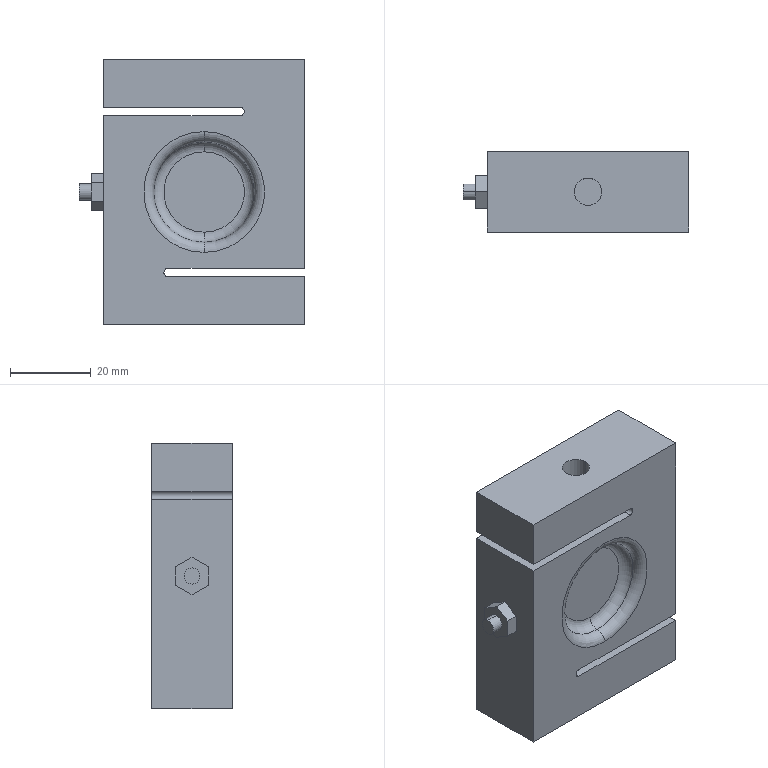Part | STEP file | Load cell JLBS-1V1.201001 | 2 solids | 34 faces | box 56 x 20 x 66 mm | volume 60086 mm3 | plane 22 | cylinder 8 | torus 4 | commonest cylinder face diameters 6.8 x4 2 x2 4 x2